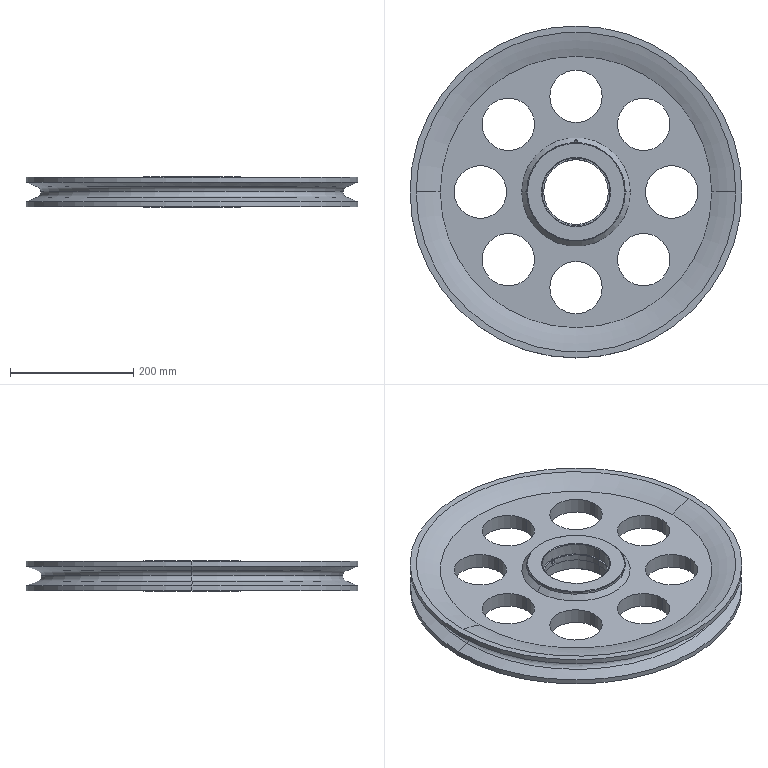Part | SolidWorks | features ICE 3, Revolution 2, Chamfer 1, CirPattern 1, CombineBodies 1 | 1 solid | 64 faces | box 538 x 538 x 50 mm | volume 4931850 mm3 | cylinder 32 | cone 16 | torus 8 | plane 8 | commonest cylinder face diameters 85 x16 110 x4 160 x4 538 x4 6 x2 105 x2